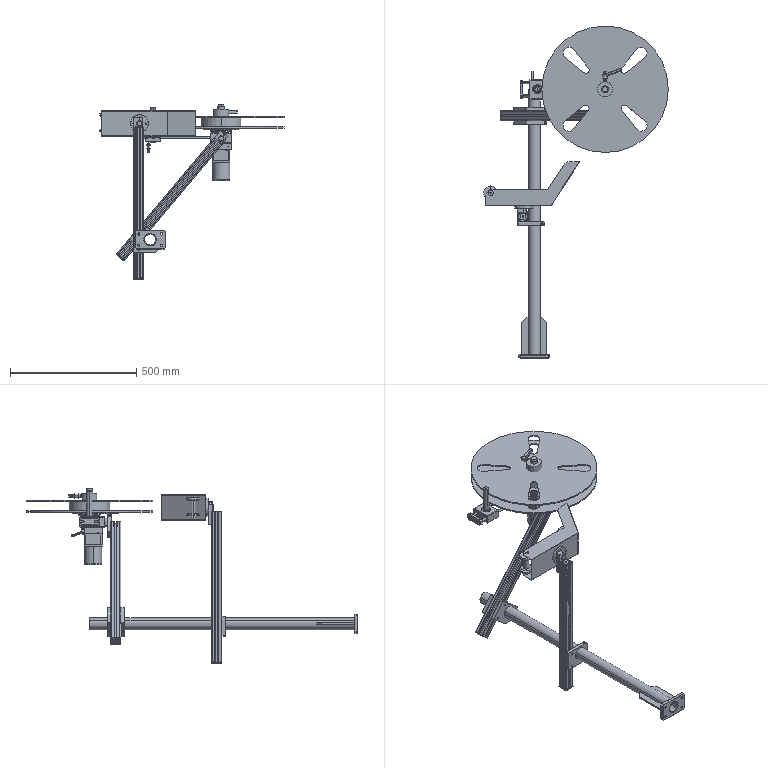Part | NX | 43 solids | 1496 faces | box 729.952 x 1312 x 692.47 mm | volume 6112875 mm3 | cylinder 582 | plane 524 | cone 293 | torus 57 | spline 30 | sphere 10 | commonest cylinder face diameters 4.2 x44 10 x39 8 x36 6.5 x28 25 x28 19 x26